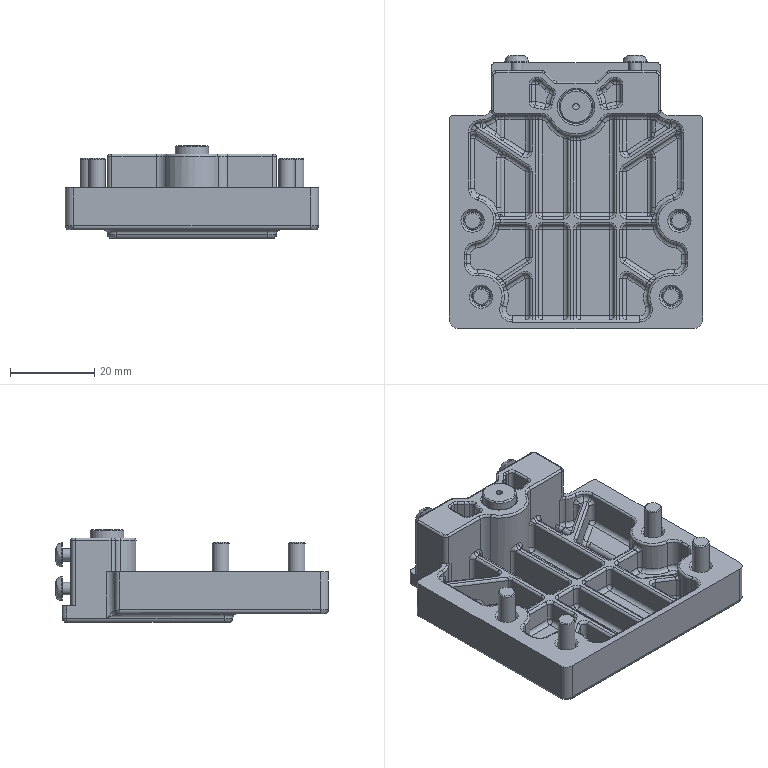Part | STEP file | BODY4_E-RAM6-S-640-ME30-C5 | 1 solid | 682 faces | box 60 x 64.65 x 22 mm | volume 24939 mm3 | cylinder 259 | plane 168 | torus 120 | sphere 64 | spline 57 | cone 14 | commonest cylinder face diameters 2 x148 1.2 x32 1 x20 5 x12 4 x8 8 x5